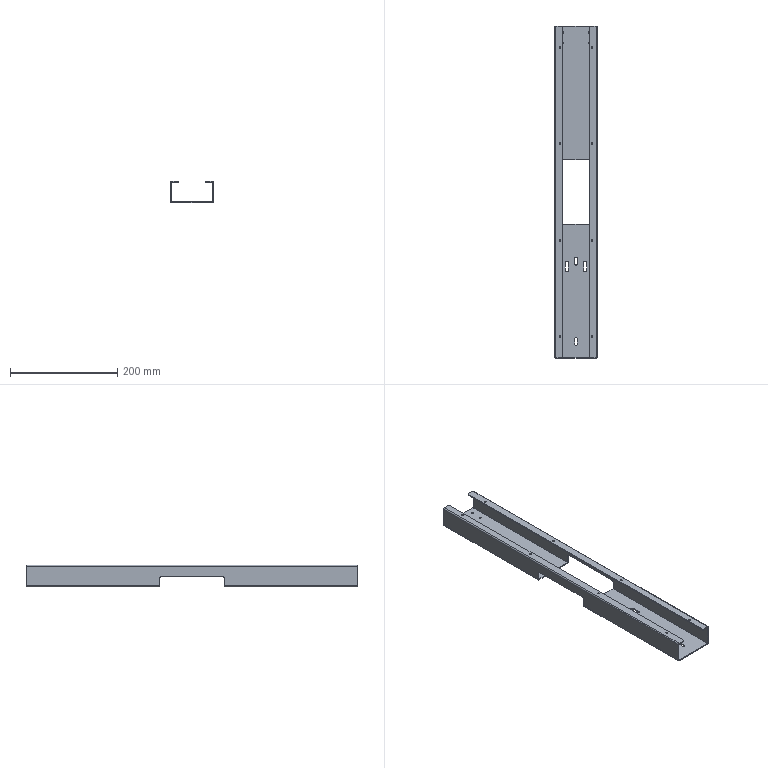Part | STEP file | 1 solid | 104 faces | box 80 x 620 x 40 mm | volume 194874 mm3 | cylinder 52 | plane 52 | commonest cylinder face diameters 3.3 x24 0.2 x6 4.2 x6 4 x4 4.5 x4 5.5 x4